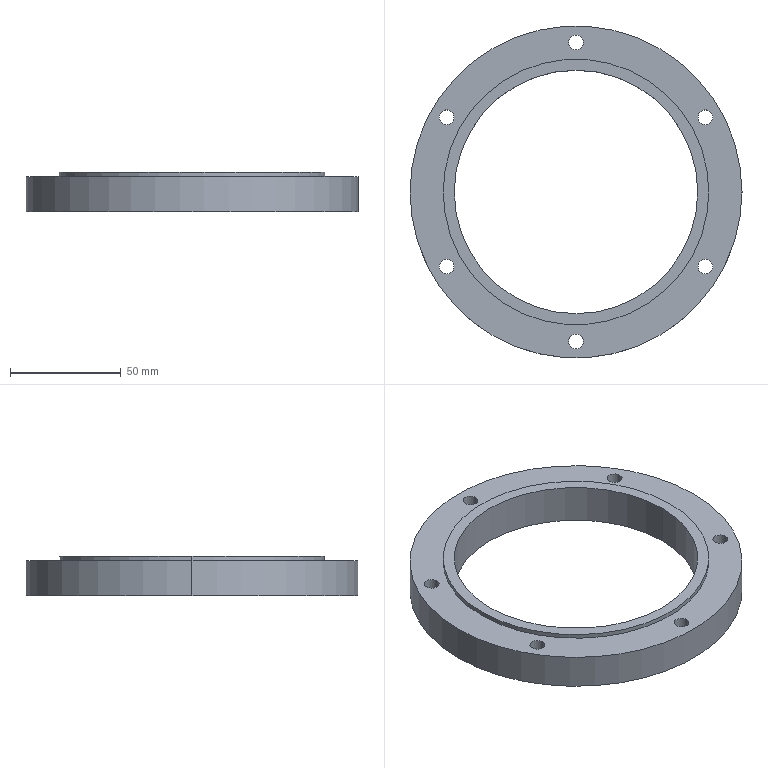Part | SolidWorks | features Extrusion 1, ICE 1 | 1 solid | 21 faces | box 150 x 150 x 18 mm | volume 130969 mm3 | cylinder 18 | plane 3 | commonest cylinder face diameters 6.65 x12 110 x2 120 x2 150 x2
STEP:
#1=CARTESIAN_POINT('',(60.,0.,18.));
#2=VERTEX_POINT('',#1);
#3=CARTESIAN_POINT('',(-60.,0.,18.));
#4=VERTEX_POINT('',#3);
#5=CARTESIAN_POINT('',(0.,0.,18.));
#6=DIRECTION('',(0.,0.,1.));
#7=DIRECTION('',(1.,0.,0.));
#8=AXIS2_PLACEMENT_3D('',#5,#6,#7);
#9=CIRCLE('',#8,60.);
#10=EDGE_CURVE('',#2,#4,#9,.T.);
#11=ORIENTED_EDGE('',*,*,#10,.F.);
#12=CARTESIAN_POINT('',(60.,0.,16.));
#13=VERTEX_POINT('',#12);
#14=CARTESIAN_POINT('',(60.,0.,18.));
#15=DIRECTION('',(0.,0.,-1.));
#16=VECTOR('',#15,1000.);
#17=LINE('',#14,#16);
#18=EDGE_CURVE('',#2,#13,#17,.T.);
#19=ORIENTED_EDGE('',*,*,#18,.T.);
#20=CARTESIAN_POINT('',(-60.,0.,16.));
#21=VERTEX_POINT('',#20);
#22=CARTESIAN_POINT('',(0.,0.,16.));
#23=DIRECTION('',(0.,0.,1.));
#24=DIRECTION('',(1.,0.,0.));
#25=AXIS2_PLACEMENT_3D('',#22,#23,#24);
#26=CIRCLE('',#25,60.);
#27=EDGE_CURVE('',#13,#21,#26,.T.);
#28=ORIENTED_EDGE('',*,*,#27,.T.);
#29=CARTESIAN_POINT('',(-60.,0.,18.));
#30=DIRECTION('',(0.,0.,-1.));
#31=VECTOR('',#30,1000.);
#32=LINE('',#29,#31);
#33=EDGE_CURVE('',#4,#21,#32,.T.);
#34=ORIENTED_EDGE('',*,*,#33,.F.);
#35=EDGE_LOOP('',(#11,#19,#28,#34));
#36=FACE_OUTER_BOUND('',#35,.T.);
#37=CARTESIAN_POINT('',(0.,0.,18.));
#38=DIRECTION('',(0.,0.,-1.));
#39=DIRECTION('',(-1.,0.,0.));
#40=AXIS2_PLACEMENT_3D('',#37,#38,#39);
#41=CYLINDRICAL_SURFACE('',#40,60.);
#42=ADVANCED_FACE('',(#36),#41,.T.);
#43=CARTESIAN_POINT('',(-61.782,33.75,16.));
#44=VERTEX_POINT('',#43);
#45=CARTESIAN_POINT('',(-55.132,33.75,16.));
#46=VERTEX_POINT('',#45);
#47=CARTESIAN_POINT('',(-58.457,33.75,16.));
#48=DIRECTION('',(0.,0.,1.));
#49=DIRECTION('',(1.,0.,0.));
#50=AXIS2_PLACEMENT_3D('',#47,#48,#49);
#51=CIRCLE('',#50,3.325);
#52=EDGE_CURVE('',#44,#46,#51,.T.);
#53=ORIENTED_EDGE('',*,*,#52,.T.);
#54=CARTESIAN_POINT('',(-55.132,33.75,0.));
#55=VERTEX_POINT('',#54);
#56=CARTESIAN_POINT('',(-55.132,33.75,16.));
#57=DIRECTION('',(0.,0.,-1.));
#58=VECTOR('',#57,1000.);
#59=LINE('',#56,#58);
#60=EDGE_CURVE('',#46,#55,#59,.T.);
#61=ORIENTED_EDGE('',*,*,#60,.T.);
#62=CARTESIAN_POINT('',(-61.782,33.75,0.));
#63=VERTEX_POINT('',#62);
#64=CARTESIAN_POINT('',(-58.457,33.75,0.));
#65=DIRECTION('',(0.,0.,1.));
#66=DIRECTION('',(1.,0.,0.));
#67=AXIS2_PLACEMENT_3D('',#64,#65,#66);
#68=CIRCLE('',#67,3.325);
#69=EDGE_CURVE('',#63,#55,#68,.T.);
#70=ORIENTED_EDGE('',*,*,#69,.F.);
#71=CARTESIAN_POINT('',(-61.782,33.75,16.));
#72=DIRECTION('',(0.,0.,-1.));
#73=VECTOR('',#72,1000.);
#74=LINE('',#71,#73);
#75=EDGE_CURVE('',#44,#63,#74,.T.);
#76=ORIENTED_EDGE('',*,*,#75,.F.);
#77=EDGE_LOOP('',(#53,#61,#70,#76));
#78=FACE_OUTER_BOUND('',#77,.T.);
#79=CARTESIAN_POINT('',(-58.457,33.75,16.));
#80=DIRECTION('',(0.,0.,-1.));
#81=DIRECTION('',(-1.,0.,0.));
#82=AXIS2_PLACEMENT_3D('',#79,#80,#81);
#83=CYLINDRICAL_SURFACE('',#82,3.325);
#84=ADVANCED_FACE('',(#78),#83,.F.);
#85=CARTESIAN_POINT('',(-61.782,-33.75,16.));
#86=VERTEX_POINT('',#85);
#87=CARTESIAN_POINT('',(-55.132,-33.75,16.));
#88=VERTEX_POINT('',#87);
#89=CARTESIAN_POINT('',(-58.457,-33.75,16.));
#90=DIRECTION('',(0.,0.,1.));
#91=DIRECTION('',(1.,0.,0.));
#92=AXIS2_PLACEMENT_3D('',#89,#90,#91);
#93=CIRCLE('',#92,3.325);
#94=EDGE_CURVE('',#86,#88,#93,.T.);
#95=ORIENTED_EDGE('',*,*,#94,.T.);
#96=CARTESIAN_POINT('',(-55.132,-33.75,0.));
#97=VERTEX_POINT('',#96);
#98=CARTESIAN_POINT('',(-55.132,-33.75,16.));
#99=DIRECTION('',(0.,0.,-1.));
#100=VECTOR('',#99,1000.);
#101=LINE('',#98,#100);
#102=EDGE_CURVE('',#88,#97,#101,.T.);
#103=ORIENTED_EDGE('',*,*,#102,.T.);
#104=CARTESIAN_POINT('',(-61.782,-33.75,0.));
#105=VERTEX_POINT('',#104);
#106=CARTESIAN_POINT('',(-58.457,-33.75,0.));
#107=DIRECTION('',(0.,0.,1.));
#108=DIRECTION('',(1.,0.,0.));
#109=AXIS2_PLACEMENT_3D('',#106,#107,#108);
#110=CIRCLE('',#109,3.325);
#111=EDGE_CURVE('',#105,#97,#110,.T.);
#112=ORIENTED_EDGE('',*,*,#111,.F.);
#113=CARTESIAN_POINT('',(-61.782,-33.75,16.));
#114=DIRECTION('',(0.,0.,-1.));
#115=VECTOR('',#114,1000.);
#116=LINE('',#113,#115);
#117=EDGE_CURVE('',#86,#105,#116,.T.);
#118=ORIENTED_EDGE('',*,*,#117,.F.);
#119=EDGE_LOOP('',(#95,#103,#112,#118));
#120=FACE_OUTER_BOUND('',#119,.T.);
#121=CARTESIAN_POINT('',(-58.457,-33.75,16.));
#122=DIRECTION('',(0.,0.,-1.));
#123=DIRECTION('',(-1.,0.,0.));
#124=AXIS2_PLACEMENT_3D('',#121,#122,#123);
#125=CYLINDRICAL_SURFACE('',#124,3.325);
#126=ADVANCED_FACE('',(#120),#125,.F.);
#127=CARTESIAN_POINT('',(-3.325,-67.5,16.));
#128=VERTEX_POINT('',#127);
#129=CARTESIAN_POINT('',(3.325,-67.5,16.));
#130=VERTEX_POINT('',#129);
#131=CARTESIAN_POINT('',(0.,-67.5,16.));
#132=DIRECTION('',(0.,0.,1.));
#133=DIRECTION('',(1.,0.,0.));
#134=AXIS2_PLACEMENT_3D('',#131,#132,#133);
#135=CIRCLE('',#134,3.325);
#136=EDGE_CURVE('',#128,#130,#135,.T.);
#137=ORIENTED_EDGE('',*,*,#136,.T.);
#138=CARTESIAN_POINT('',(3.325,-67.5,0.));
#139=VERTEX_POINT('',#138);
#140=CARTESIAN_POINT('',(3.325,-67.5,16.));
#141=DIRECTION('',(0.,0.,-1.));
#142=VECTOR('',#141,1000.);
#143=LINE('',#140,#142);
#144=EDGE_CURVE('',#130,#139,#143,.T.);
#145=ORIENTED_EDGE('',*,*,#144,.T.);
#146=CARTESIAN_POINT('',(-3.325,-67.5,0.));
#147=VERTEX_POINT('',#146);
#148=CARTESIAN_POINT('',(0.,-67.5,0.));
#149=DIRECTION('',(0.,0.,1.));
#150=DIRECTION('',(1.,0.,0.));
#151=AXIS2_PLACEMENT_3D('',#148,#149,#150);
#152=CIRCLE('',#151,3.325);
#153=EDGE_CURVE('',#147,#139,#152,.T.);
#154=ORIENTED_EDGE('',*,*,#153,.F.);
#155=CARTESIAN_POINT('',(-3.325,-67.5,16.));
#156=DIRECTION('',(0.,0.,-1.));
#157=VECTOR('',#156,1000.);
#158=LINE('',#155,#157);
#159=EDGE_CURVE('',#128,#147,#158,.T.);
#160=ORIENTED_EDGE('',*,*,#159,.F.);
#161=EDGE_LOOP('',(#137,#145,#154,#160));
#162=FACE_OUTER_BOUND('',#161,.T.);
#163=CARTESIAN_POINT('',(0.,-67.5,16.));
#164=DIRECTION('',(0.,0.,-1.));
#165=DIRECTION('',(-1.,0.,0.));
#166=AXIS2_PLACEMENT_3D('',#163,#164,#165);
#167=CYLINDRICAL_SURFACE('',#166,3.325);
#168=ADVANCED_FACE('',(#162),#167,.F.);
#169=CARTESIAN_POINT('',(55.132,-33.75,16.));
#170=VERTEX_POINT('',#169);
#171=CARTESIAN_POINT('',(61.782,-33.75,16.));
#172=VERTEX_POINT('',#171);
#173=CARTESIAN_POINT('',(58.457,-33.75,16.));
#174=DIRECTION('',(0.,0.,1.));
#175=DIRECTION('',(1.,0.,0.));
#176=AXIS2_PLACEMENT_3D('',#173,#174,#175);
#177=CIRCLE('',#176,3.325);
#178=EDGE_CURVE('',#170,#172,#177,.T.);
#179=ORIENTED_EDGE('',*,*,#178,.T.);
#180=CARTESIAN_POINT('',(61.782,-33.75,0.));
#181=VERTEX_POINT('',#180);
#182=CARTESIAN_POINT('',(61.782,-33.75,16.));
#183=DIRECTION('',(0.,0.,-1.));
#184=VECTOR('',#183,1000.);
#185=LINE('',#182,#184);
#186=EDGE_CURVE('',#172,#181,#185,.T.);
#187=ORIENTED_EDGE('',*,*,#186,.T.);
#188=CARTESIAN_POINT('',(55.132,-33.75,0.));
#189=VERTEX_POINT('',#188);
#190=CARTESIAN_POINT('',(58.457,-33.75,0.));
#191=DIRECTION('',(0.,0.,1.));
#192=DIRECTION('',(1.,0.,0.));
#193=AXIS2_PLACEMENT_3D('',#190,#191,#192);
#194=CIRCLE('',#193,3.325);
#195=EDGE_CURVE('',#189,#181,#194,.T.);
#196=ORIENTED_EDGE('',*,*,#195,.F.);
#197=CARTESIAN_POINT('',(55.132,-33.75,16.));
#198=DIRECTION('',(0.,0.,-1.));
#199=VECTOR('',#198,1000.);
#200=LINE('',#197,#199);
#201=EDGE_CURVE('',#170,#189,#200,.T.);
#202=ORIENTED_EDGE('',*,*,#201,.F.);
#203=EDGE_LOOP('',(#179,#187,#196,#202));
#204=FACE_OUTER_BOUND('',#203,.T.);
#205=CARTESIAN_POINT('',(58.457,-33.75,16.));
#206=DIRECTION('',(0.,0.,-1.));
#207=DIRECTION('',(-1.,0.,0.));
#208=AXIS2_PLACEMENT_3D('',#205,#206,#207);
#209=CYLINDRICAL_SURFACE('',#208,3.325);
#210=ADVANCED_FACE('',(#204),#209,.F.);
#211=CARTESIAN_POINT('',(55.132,33.75,16.));
#212=VERTEX_POINT('',#211);
#213=CARTESIAN_POINT('',(61.782,33.75,16.));
#214=VERTEX_POINT('',#213);
#215=CARTESIAN_POINT('',(58.457,33.75,16.));
#216=DIRECTION('',(0.,0.,1.));
#217=DIRECTION('',(1.,0.,0.));
#218=AXIS2_PLACEMENT_3D('',#215,#216,#217);
#219=CIRCLE('',#218,3.325);
#220=EDGE_CURVE('',#212,#214,#219,.T.);
#221=ORIENTED_EDGE('',*,*,#220,.T.);
#222=CARTESIAN_POINT('',(61.782,33.75,0.));
#223=VERTEX_POINT('',#222);
#224=CARTESIAN_POINT('',(61.782,33.75,16.));
#225=DIRECTION('',(0.,0.,-1.));
#226=VECTOR('',#225,1000.);
#227=LINE('',#224,#226);
#228=EDGE_CURVE('',#214,#223,#227,.T.);
#229=ORIENTED_EDGE('',*,*,#228,.T.);
#230=CARTESIAN_POINT('',(55.132,33.75,0.));
#231=VERTEX_POINT('',#230);
#232=CARTESIAN_POINT('',(58.457,33.75,0.));
#233=DIRECTION('',(0.,0.,1.));
#234=DIRECTION('',(1.,0.,0.));
#235=AXIS2_PLACEMENT_3D('',#232,#233,#234);
#236=CIRCLE('',#235,3.325);
#237=EDGE_CURVE('',#231,#223,#236,.T.);
#238=ORIENTED_EDGE('',*,*,#237,.F.);
#239=CARTESIAN_POINT('',(55.132,33.75,16.));
#240=DIRECTION('',(0.,0.,-1.));
#241=VECTOR('',#240,1000.);
#242=LINE('',#239,#241);
#243=EDGE_CURVE('',#212,#231,#242,.T.);
#244=ORIENTED_EDGE('',*,*,#243,.F.);
#245=EDGE_LOOP('',(#221,#229,#238,#244));
#246=FACE_OUTER_BOUND('',#245,.T.);
#247=CARTESIAN_POINT('',(58.457,33.75,16.));
#248=DIRECTION('',(0.,0.,-1.));
#249=DIRECTION('',(-1.,0.,0.));
#250=AXIS2_PLACEMENT_3D('',#247,#248,#249);
#251=CYLINDRICAL_SURFACE('',#250,3.325);
#252=ADVANCED_FACE('',(#246),#251,.F.);
#253=CARTESIAN_POINT('',(-3.325,67.5,16.));
#254=VERTEX_POINT('',#253);
#255=CARTESIAN_POINT('',(3.325,67.5,16.));
#256=VERTEX_POINT('',#255);
#257=CARTESIAN_POINT('',(0.,67.5,16.));
#258=DIRECTION('',(0.,0.,1.));
#259=DIRECTION('',(1.,0.,0.));
#260=AXIS2_PLACEMENT_3D('',#257,#258,#259);
#261=CIRCLE('',#260,3.325);
#262=EDGE_CURVE('',#254,#256,#261,.T.);
#263=ORIENTED_EDGE('',*,*,#262,.T.);
#264=CARTESIAN_POINT('',(3.325,67.5,0.));
#265=VERTEX_POINT('',#264);
#266=CARTESIAN_POINT('',(3.325,67.5,16.));
#267=DIRECTION('',(0.,0.,-1.));
#268=VECTOR('',#267,1000.);
#269=LINE('',#266,#268);
#270=EDGE_CURVE('',#256,#265,#269,.T.);
#271=ORIENTED_EDGE('',*,*,#270,.T.);
#272=CARTESIAN_POINT('',(-3.325,67.5,0.));
#273=VERTEX_POINT('',#272);
#274=CARTESIAN_POINT('',(0.,67.5,0.));
#275=DIRECTION('',(0.,0.,1.));
#276=DIRECTION('',(1.,0.,0.));
#277=AXIS2_PLACEMENT_3D('',#274,#275,#276);
#278=CIRCLE('',#277,3.325);
#279=EDGE_CURVE('',#273,#265,#278,.T.);
#280=ORIENTED_EDGE('',*,*,#279,.F.);
#281=CARTESIAN_POINT('',(-3.325,67.5,16.));
#282=DIRECTION('',(0.,0.,-1.));
#283=VECTOR('',#282,1000.);
#284=LINE('',#281,#283);
#285=EDGE_CURVE('',#254,#273,#284,.T.);
#286=ORIENTED_EDGE('',*,*,#285,.F.);
#287=EDGE_LOOP('',(#263,#271,#280,#286));
#288=FACE_OUTER_BOUND('',#287,.T.);
#289=CARTESIAN_POINT('',(0.,67.5,16.));
#290=DIRECTION('',(0.,0.,-1.));
#291=DIRECTION('',(-1.,0.,0.));
#292=AXIS2_PLACEMENT_3D('',#289,#290,#291);
#293=CYLINDRICAL_SURFACE('',#292,3.325);
#294=ADVANCED_FACE('',(#288),#293,.F.);
#295=CARTESIAN_POINT('',(-55.,0.,18.));
#296=VERTEX_POINT('',#295);
#297=CARTESIAN_POINT('',(55.,0.,18.));
#298=VERTEX_POINT('',#297);
#299=CARTESIAN_POINT('',(0.,0.,18.));
#300=DIRECTION('',(0.,0.,1.));
#301=DIRECTION('',(1.,0.,0.));
#302=AXIS2_PLACEMENT_3D('',#299,#300,#301);
#303=CIRCLE('',#302,55.);
#304=EDGE_CURVE('',#296,#298,#303,.T.);
#305=ORIENTED_EDGE('',*,*,#304,.T.);
#306=CARTESIAN_POINT('',(55.,0.,0.));
#307=VERTEX_POINT('',#306);
#308=CARTESIAN_POINT('',(55.,0.,16.));
#309=DIRECTION('',(0.,0.,-1.));
#310=VECTOR('',#309,1000.);
#311=LINE('',#308,#310);
#312=EDGE_CURVE('',#298,#307,#311,.T.);
#313=ORIENTED_EDGE('',*,*,#312,.T.);
#314=CARTESIAN_POINT('',(-55.,0.,0.));
#315=VERTEX_POINT('',#314);
#316=CARTESIAN_POINT('',(0.,0.,0.));
#317=DIRECTION('',(0.,0.,1.));
#318=DIRECTION('',(1.,0.,0.));
#319=AXIS2_PLACEMENT_3D('',#316,#317,#318);
#320=CIRCLE('',#319,55.);
#321=EDGE_CURVE('',#315,#307,#320,.T.);
#322=ORIENTED_EDGE('',*,*,#321,.F.);
#323=CARTESIAN_POINT('',(-55.,0.,16.));
#324=DIRECTION('',(0.,0.,-1.));
#325=VECTOR('',#324,1000.);
#326=LINE('',#323,#325);
#327=EDGE_CURVE('',#296,#315,#326,.T.);
#328=ORIENTED_EDGE('',*,*,#327,.F.);
#329=EDGE_LOOP('',(#305,#313,#322,#328));
#330=FACE_OUTER_BOUND('',#329,.T.);
#331=CARTESIAN_POINT('',(0.,0.,16.));
#332=DIRECTION('',(0.,0.,-1.));
#333=DIRECTION('',(-1.,0.,0.));
#334=AXIS2_PLACEMENT_3D('',#331,#332,#333);
#335=CYLINDRICAL_SURFACE('',#334,55.);
#336=ADVANCED_FACE('',(#330),#335,.F.);
#337=CARTESIAN_POINT('',(75.,0.,16.));
#338=VERTEX_POINT('',#337);
#339=CARTESIAN_POINT('',(-75.,0.,16.));
#340=VERTEX_POINT('',#339);
#341=CARTESIAN_POINT('',(0.,0.,16.));
#342=DIRECTION('',(0.,0.,1.));
#343=DIRECTION('',(1.,0.,0.));
#344=AXIS2_PLACEMENT_3D('',#341,#342,#343);
#345=CIRCLE('',#344,75.);
#346=EDGE_CURVE('',#338,#340,#345,.T.);
#347=ORIENTED_EDGE('',*,*,#346,.F.);
#348=CARTESIAN_POINT('',(75.,0.,0.));
#349=VERTEX_POINT('',#348);
#350=CARTESIAN_POINT('',(75.,0.,16.));
#351=DIRECTION('',(0.,0.,-1.));
#352=VECTOR('',#351,1000.);
#353=LINE('',#350,#352);
#354=EDGE_CURVE('',#338,#349,#353,.T.);
#355=ORIENTED_EDGE('',*,*,#354,.T.);
#356=CARTESIAN_POINT('',(-75.,0.,0.));
#357=VERTEX_POINT('',#356);
#358=CARTESIAN_POINT('',(0.,0.,0.));
#359=DIRECTION('',(0.,0.,1.));
#360=DIRECTION('',(1.,0.,0.));
#361=AXIS2_PLACEMENT_3D('',#358,#359,#360);
#362=CIRCLE('',#361,75.);
#363=EDGE_CURVE('',#349,#357,#362,.T.);
#364=ORIENTED_EDGE('',*,*,#363,.T.);
#365=CARTESIAN_POINT('',(-75.,0.,16.));
#366=DIRECTION('',(0.,0.,-1.));
#367=VECTOR('',#366,1000.);
#368=LINE('',#365,#367);
#369=EDGE_CURVE('',#340,#357,#368,.T.);
#370=ORIENTED_EDGE('',*,*,#369,.F.);
#371=EDGE_LOOP('',(#347,#355,#364,#370));
#372=FACE_OUTER_BOUND('',#371,.T.);
#373=CARTESIAN_POINT('',(0.,0.,16.));
#374=DIRECTION('',(0.,0.,-1.));
#375=DIRECTION('',(-1.,0.,0.));
#376=AXIS2_PLACEMENT_3D('',#373,#374,#375);
#377=CYLINDRICAL_SURFACE('',#376,75.);
#378=ADVANCED_FACE('',(#372),#377,.T.);
#379=ORIENTED_EDGE('',*,*,#52,.F.);
#380=CARTESIAN_POINT('',(-58.457,33.75,16.));
#381=DIRECTION('',(0.,0.,1.));
#382=DIRECTION('',(1.,0.,0.));
#383=AXIS2_PLACEMENT_3D('',#380,#381,#382);
#384=CIRCLE('',#383,3.325);
#385=EDGE_CURVE('',#46,#44,#384,.T.);
#386=ORIENTED_EDGE('',*,*,#385,.F.);
#387=EDGE_LOOP('',(#379,#386));
#388=FACE_BOUND('',#387,.T.);
#389=ORIENTED_EDGE('',*,*,#136,.F.);
#390=CARTESIAN_POINT('',(0.,-67.5,16.));
#391=DIRECTION('',(0.,0.,1.));
#392=DIRECTION('',(1.,0.,0.));
#393=AXIS2_PLACEMENT_3D('',#390,#391,#392);
#394=CIRCLE('',#393,3.325);
#395=EDGE_CURVE('',#130,#128,#394,.T.);
#396=ORIENTED_EDGE('',*,*,#395,.F.);
#397=EDGE_LOOP('',(#389,#396));
#398=FACE_BOUND('',#397,.T.);
#399=ORIENTED_EDGE('',*,*,#220,.F.);
#400=CARTESIAN_POINT('',(58.457,33.75,16.));
#401=DIRECTION('',(0.,0.,1.));
#402=DIRECTION('',(1.,0.,0.));
#403=AXIS2_PLACEMENT_3D('',#400,#401,#402);
#404=CIRCLE('',#403,3.325);
#405=EDGE_CURVE('',#214,#212,#404,.T.);
#406=ORIENTED_EDGE('',*,*,#405,.F.);
#407=EDGE_LOOP('',(#399,#406));
#408=FACE_BOUND('',#407,.T.);
#409=CARTESIAN_POINT('',(0.,0.,16.));
#410=DIRECTION('',(0.,0.,1.));
#411=DIRECTION('',(1.,0.,0.));
#412=AXIS2_PLACEMENT_3D('',#409,#410,#411);
#413=CIRCLE('',#412,75.);
#414=EDGE_CURVE('',#340,#338,#413,.T.);
#415=ORIENTED_EDGE('',*,*,#414,.T.);
#416=ORIENTED_EDGE('',*,*,#346,.T.);
#417=EDGE_LOOP('',(#415,#416));
#418=FACE_OUTER_BOUND('',#417,.T.);
#419=ORIENTED_EDGE('',*,*,#262,.F.);
#420=CARTESIAN_POINT('',(0.,67.5,16.));
#421=DIRECTION('',(0.,0.,1.));
#422=DIRECTION('',(1.,0.,0.));
#423=AXIS2_PLACEMENT_3D('',#420,#421,#422);
#424=CIRCLE('',#423,3.325);
#425=EDGE_CURVE('',#256,#254,#424,.T.);
#426=ORIENTED_EDGE('',*,*,#425,.F.);
#427=EDGE_LOOP('',(#419,#426));
#428=FACE_BOUND('',#427,.T.);
#429=ORIENTED_EDGE('',*,*,#178,.F.);
#430=CARTESIAN_POINT('',(58.457,-33.75,16.));
#431=DIRECTION('',(0.,0.,1.));
#432=DIRECTION('',(1.,0.,0.));
#433=AXIS2_PLACEMENT_3D('',#430,#431,#432);
#434=CIRCLE('',#433,3.325);
#435=EDGE_CURVE('',#172,#170,#434,.T.);
#436=ORIENTED_EDGE('',*,*,#435,.F.);
#437=EDGE_LOOP('',(#429,#436));
#438=FACE_BOUND('',#437,.T.);
#439=ORIENTED_EDGE('',*,*,#94,.F.);
#440=CARTESIAN_POINT('',(-58.457,-33.75,16.));
#441=DIRECTION('',(0.,0.,1.));
#442=DIRECTION('',(1.,0.,0.));
#443=AXIS2_PLACEMENT_3D('',#440,#441,#442);
#444=CIRCLE('',#443,3.325);
#445=EDGE_CURVE('',#88,#86,#444,.T.);
#446=ORIENTED_EDGE('',*,*,#445,.F.);
#447=EDGE_LOOP('',(#439,#446));
#448=FACE_BOUND('',#447,.T.);
#449=CARTESIAN_POINT('',(0.,0.,16.));
#450=DIRECTION('',(0.,0.,1.));
#451=DIRECTION('',(1.,0.,0.));
#452=AXIS2_PLACEMENT_3D('',#449,#450,#451);
#453=CIRCLE('',#452,60.);
#454=EDGE_CURVE('',#21,#13,#453,.T.);
#455=ORIENTED_EDGE('',*,*,#454,.F.);
#456=ORIENTED_EDGE('',*,*,#27,.F.);
#457=EDGE_LOOP('',(#455,#456));
#458=FACE_BOUND('',#457,.T.);
#459=CARTESIAN_POINT('',(0.,0.,16.));
#460=DIRECTION('',(0.,0.,1.));
#461=DIRECTION('',(1.,0.,0.));
#462=AXIS2_PLACEMENT_3D('',#459,#460,#461);
#463=PLANE('',#462);
#464=ADVANCED_FACE('',(#388,#398,#408,#418,#428,#438,#448,#458),#463,.T.);
#465=CARTESIAN_POINT('',(0.,0.,0.));
#466=DIRECTION('',(0.,0.,1.));
#467=DIRECTION('',(1.,0.,0.));
#468=AXIS2_PLACEMENT_3D('',#465,#466,#467);
#469=CIRCLE('',#468,75.);
#470=EDGE_CURVE('',#357,#349,#469,.T.);
#471=ORIENTED_EDGE('',*,*,#470,.F.);
#472=ORIENTED_EDGE('',*,*,#363,.F.);
#473=EDGE_LOOP('',(#471,#472));
#474=FACE_OUTER_BOUND('',#473,.T.);
#475=ORIENTED_EDGE('',*,*,#321,.T.);
#476=CARTESIAN_POINT('',(0.,0.,0.));
#477=DIRECTION('',(0.,0.,1.));
#478=DIRECTION('',(1.,0.,0.));
#479=AXIS2_PLACEMENT_3D('',#476,#477,#478);
#480=CIRCLE('',#479,55.);
#481=EDGE_CURVE('',#307,#315,#480,.T.);
#482=ORIENTED_EDGE('',*,*,#481,.T.);
#483=EDGE_LOOP('',(#475,#482));
#484=FACE_BOUND('',#483,.T.);
#485=ORIENTED_EDGE('',*,*,#279,.T.);
#486=CARTESIAN_POINT('',(0.,67.5,0.));
#487=DIRECTION('',(0.,0.,1.));
#488=DIRECTION('',(1.,0.,0.));
#489=AXIS2_PLACEMENT_3D('',#486,#487,#488);
#490=CIRCLE('',#489,3.325);
#491=EDGE_CURVE('',#265,#273,#490,.T.);
#492=ORIENTED_EDGE('',*,*,#491,.T.);
#493=EDGE_LOOP('',(#485,#492));
#494=FACE_BOUND('',#493,.T.);
#495=ORIENTED_EDGE('',*,*,#237,.T.);
#496=CARTESIAN_POINT('',(58.457,33.75,0.));
#497=DIRECTION('',(0.,0.,1.));
#498=DIRECTION('',(1.,0.,0.));
#499=AXIS2_PLACEMENT_3D('',#496,#497,#498);
#500=CIRCLE('',#499,3.325);
#501=EDGE_CURVE('',#223,#231,#500,.T.);
#502=ORIENTED_EDGE('',*,*,#501,.T.);
#503=EDGE_LOOP('',(#495,#502));
#504=FACE_BOUND('',#503,.T.);
#505=ORIENTED_EDGE('',*,*,#195,.T.);
#506=CARTESIAN_POINT('',(58.457,-33.75,0.));
#507=DIRECTION('',(0.,0.,1.));
#508=DIRECTION('',(1.,0.,0.));
#509=AXIS2_PLACEMENT_3D('',#506,#507,#508);
#510=CIRCLE('',#509,3.325);
#511=EDGE_CURVE('',#181,#189,#510,.T.);
#512=ORIENTED_EDGE('',*,*,#511,.T.);
#513=EDGE_LOOP('',(#505,#512));
#514=FACE_BOUND('',#513,.T.);
#515=ORIENTED_EDGE('',*,*,#153,.T.);
#516=CARTESIAN_POINT('',(0.,-67.5,0.));
#517=DIRECTION('',(0.,0.,1.));
#518=DIRECTION('',(1.,0.,0.));
#519=AXIS2_PLACEMENT_3D('',#516,#517,#518);
#520=CIRCLE('',#519,3.325);
#521=EDGE_CURVE('',#139,#147,#520,.T.);
#522=ORIENTED_EDGE('',*,*,#521,.T.);
#523=EDGE_LOOP('',(#515,#522));
#524=FACE_BOUND('',#523,.T.);
#525=ORIENTED_EDGE('',*,*,#111,.T.);
#526=CARTESIAN_POINT('',(-58.457,-33.75,0.));
#527=DIRECTION('',(0.,0.,1.));
#528=DIRECTION('',(1.,0.,0.));
#529=AXIS2_PLACEMENT_3D('',#526,#527,#528);
#530=CIRCLE('',#529,3.325);
#531=EDGE_CURVE('',#97,#105,#530,.T.);
#532=ORIENTED_EDGE('',*,*,#531,.T.);
#533=EDGE_LOOP('',(#525,#532));
#534=FACE_BOUND('',#533,.T.);
#535=ORIENTED_EDGE('',*,*,#69,.T.);
#536=CARTESIAN_POINT('',(-58.457,33.75,0.));
#537=DIRECTION('',(0.,0.,1.));
#538=DIRECTION('',(1.,0.,0.));
#539=AXIS2_PLACEMENT_3D('',#536,#537,#538);
#540=CIRCLE('',#539,3.325);
#541=EDGE_CURVE('',#55,#63,#540,.T.);
#542=ORIENTED_EDGE('',*,*,#541,.T.);
#543=EDGE_LOOP('',(#535,#542));
#544=FACE_BOUND('',#543,.T.);
#545=CARTESIAN_POINT('',(0.,0.,0.));
#546=DIRECTION('',(0.,0.,1.));
#547=DIRECTION('',(1.,0.,0.));
#548=AXIS2_PLACEMENT_3D('',#545,#546,#547);
#549=PLANE('',#548);
#550=ADVANCED_FACE('',(#474,#484,#494,#504,#514,#524,#534,#544),#549,.F.);
#551=ORIENTED_EDGE('',*,*,#354,.F.);
#552=ORIENTED_EDGE('',*,*,#414,.F.);
#553=ORIENTED_EDGE('',*,*,#369,.T.);
#554=ORIENTED_EDGE('',*,*,#470,.T.);
#555=EDGE_LOOP('',(#551,#552,#553,#554));
#556=FACE_OUTER_BOUND('',#555,.T.);
#557=CARTESIAN_POINT('',(0.,0.,16.));
#558=DIRECTION('',(0.,0.,-1.));
#559=DIRECTION('',(-1.,0.,0.));
#560=AXIS2_PLACEMENT_3D('',#557,#558,#559);
#561=CYLINDRICAL_SURFACE('',#560,75.);
#562=ADVANCED_FACE('',(#556),#561,.T.);
#563=ORIENTED_EDGE('',*,*,#312,.F.);
#564=CARTESIAN_POINT('',(0.,0.,18.));
#565=DIRECTION('',(0.,0.,1.));
#566=DIRECTION('',(1.,0.,0.));
#567=AXIS2_PLACEMENT_3D('',#564,#565,#566);
#568=CIRCLE('',#567,55.);
#569=EDGE_CURVE('',#298,#296,#568,.T.);
#570=ORIENTED_EDGE('',*,*,#569,.T.);
#571=ORIENTED_EDGE('',*,*,#327,.T.);
#572=ORIENTED_EDGE('',*,*,#481,.F.);
#573=EDGE_LOOP('',(#563,#570,#571,#572));
#574=FACE_OUTER_BOUND('',#573,.T.);
#575=CARTESIAN_POINT('',(0.,0.,16.));
#576=DIRECTION('',(0.,0.,-1.));
#577=DIRECTION('',(-1.,0.,0.));
#578=AXIS2_PLACEMENT_3D('',#575,#576,#577);
#579=CYLINDRICAL_SURFACE('',#578,55.);
#580=ADVANCED_FACE('',(#574),#579,.F.);
#581=ORIENTED_EDGE('',*,*,#270,.F.);
#582=ORIENTED_EDGE('',*,*,#425,.T.);
#583=ORIENTED_EDGE('',*,*,#285,.T.);
#584=ORIENTED_EDGE('',*,*,#491,.F.);
#585=EDGE_LOOP('',(#581,#582,#583,#584));
#586=FACE_OUTER_BOUND('',#585,.T.);
#587=CARTESIAN_POINT('',(0.,67.5,16.));
#588=DIRECTION('',(0.,0.,-1.));
#589=DIRECTION('',(-1.,0.,0.));
#590=AXIS2_PLACEMENT_3D('',#587,#588,#589);
#591=CYLINDRICAL_SURFACE('',#590,3.325);
#592=ADVANCED_FACE('',(#586),#591,.F.);
#593=ORIENTED_EDGE('',*,*,#228,.F.);
#594=ORIENTED_EDGE('',*,*,#405,.T.);
#595=ORIENTED_EDGE('',*,*,#243,.T.);
#596=ORIENTED_EDGE('',*,*,#501,.F.);
#597=EDGE_LOOP('',(#593,#594,#595,#596));
#598=FACE_OUTER_BOUND('',#597,.T.);
#599=CARTESIAN_POINT('',(58.457,33.75,16.));
#600=DIRECTION('',(0.,0.,-1.));
#601=DIRECTION('',(-1.,0.,0.));
#602=AXIS2_PLACEMENT_3D('',#599,#600,#601);
#603=CYLINDRICAL_SURFACE('',#602,3.325);
#604=ADVANCED_FACE('',(#598),#603,.F.);
#605=ORIENTED_EDGE('',*,*,#186,.F.);
#606=ORIENTED_EDGE('',*,*,#435,.T.);
#607=ORIENTED_EDGE('',*,*,#201,.T.);
#608=ORIENTED_EDGE('',*,*,#511,.F.);
#609=EDGE_LOOP('',(#605,#606,#607,#608));
#610=FACE_OUTER_BOUND('',#609,.T.);
#611=CARTESIAN_POINT('',(58.457,-33.75,16.));
#612=DIRECTION('',(0.,0.,-1.));
#613=DIRECTION('',(-1.,0.,0.));
#614=AXIS2_PLACEMENT_3D('',#611,#612,#613);
#615=CYLINDRICAL_SURFACE('',#614,3.325);
#616=ADVANCED_FACE('',(#610),#615,.F.);
#617=ORIENTED_EDGE('',*,*,#144,.F.);
#618=ORIENTED_EDGE('',*,*,#395,.T.);
#619=ORIENTED_EDGE('',*,*,#159,.T.);
#620=ORIENTED_EDGE('',*,*,#521,.F.);
#621=EDGE_LOOP('',(#617,#618,#619,#620));
#622=FACE_OUTER_BOUND('',#621,.T.);
#623=CARTESIAN_POINT('',(0.,-67.5,16.));
#624=DIRECTION('',(0.,0.,-1.));
#625=DIRECTION('',(-1.,0.,0.));
#626=AXIS2_PLACEMENT_3D('',#623,#624,#625);
#627=CYLINDRICAL_SURFACE('',#626,3.325);
#628=ADVANCED_FACE('',(#622),#627,.F.);
#629=ORIENTED_EDGE('',*,*,#102,.F.);
#630=ORIENTED_EDGE('',*,*,#445,.T.);
#631=ORIENTED_EDGE('',*,*,#117,.T.);
#632=ORIENTED_EDGE('',*,*,#531,.F.);
#633=EDGE_LOOP('',(#629,#630,#631,#632));
#634=FACE_OUTER_BOUND('',#633,.T.);
#635=CARTESIAN_POINT('',(-58.457,-33.75,16.));
#636=DIRECTION('',(0.,0.,-1.));
#637=DIRECTION('',(-1.,0.,0.));
#638=AXIS2_PLACEMENT_3D('',#635,#636,#637);
#639=CYLINDRICAL_SURFACE('',#638,3.325);
#640=ADVANCED_FACE('',(#634),#639,.F.);
#641=ORIENTED_EDGE('',*,*,#60,.F.);
#642=ORIENTED_EDGE('',*,*,#385,.T.);
#643=ORIENTED_EDGE('',*,*,#75,.T.);
#644=ORIENTED_EDGE('',*,*,#541,.F.);
#645=EDGE_LOOP('',(#641,#642,#643,#644));
#646=FACE_OUTER_BOUND('',#645,.T.);
#647=CARTESIAN_POINT('',(-58.457,33.75,16.));
#648=DIRECTION('',(0.,0.,-1.));
#649=DIRECTION('',(-1.,0.,0.));
#650=AXIS2_PLACEMENT_3D('',#647,#648,#649);
#651=CYLINDRICAL_SURFACE('',#650,3.325);
#652=ADVANCED_FACE('',(#646),#651,.F.);
#653=CARTESIAN_POINT('',(0.,0.,18.));
#654=DIRECTION('',(0.,0.,1.));
#655=DIRECTION('',(1.,0.,0.));
#656=AXIS2_PLACEMENT_3D('',#653,#654,#655);
#657=CIRCLE('',#656,60.);
#658=EDGE_CURVE('',#4,#2,#657,.T.);
#659=ORIENTED_EDGE('',*,*,#658,.T.);
#660=ORIENTED_EDGE('',*,*,#10,.T.);
#661=EDGE_LOOP('',(#659,#660));
#662=FACE_OUTER_BOUND('',#661,.T.);
#663=ORIENTED_EDGE('',*,*,#304,.F.);
#664=ORIENTED_EDGE('',*,*,#569,.F.);
#665=EDGE_LOOP('',(#663,#664));
#666=FACE_BOUND('',#665,.T.);
#667=CARTESIAN_POINT('',(0.,0.,18.));
#668=DIRECTION('',(0.,0.,1.));
#669=DIRECTION('',(1.,0.,0.));
#670=AXIS2_PLACEMENT_3D('',#667,#668,#669);
#671=PLANE('',#670);
#672=ADVANCED_FACE('',(#662,#666),#671,.T.);
#673=ORIENTED_EDGE('',*,*,#18,.F.);
#674=ORIENTED_EDGE('',*,*,#658,.F.);
#675=ORIENTED_EDGE('',*,*,#33,.T.);
#676=ORIENTED_EDGE('',*,*,#454,.T.);
#677=EDGE_LOOP('',(#673,#674,#675,#676));
#678=FACE_OUTER_BOUND('',#677,.T.);
#679=CARTESIAN_POINT('',(0.,0.,18.));
#680=DIRECTION('',(0.,0.,-1.));
#681=DIRECTION('',(-1.,0.,0.));
#682=AXIS2_PLACEMENT_3D('',#679,#680,#681);
#683=CYLINDRICAL_SURFACE('',#682,60.);
#684=ADVANCED_FACE('',(#678),#683,.T.);
#685=CLOSED_SHELL('',(#42,#84,#126,#168,#210,#252,#294,#336,#378,#464,#550,#562,#580,#592,#604,#616,#628,#640,#652,#672,#684));
#686=MANIFOLD_SOLID_BREP('',#685);
#687=CARTESIAN_POINT('',(0.,0.,0.));
#688=DIRECTION('',(0.,0.,1.));
#689=DIRECTION('',(1.,0.,0.));
#690=AXIS2_PLACEMENT_3D('',#687,#688,#689);
#691=(LENGTH_UNIT()NAMED_UNIT(*)SI_UNIT(.MILLI.,.METRE.));
#692=UNCERTAINTY_MEASURE_WITH_UNIT(LENGTH_MEASURE(0.00001),#691,'','');
#693=(NAMED_UNIT(*)PLANE_ANGLE_UNIT()SI_UNIT($,.RADIAN.));
#694=(NAMED_UNIT(*)SI_UNIT($,.STERADIAN.)SOLID_ANGLE_UNIT());
#695=(GEOMETRIC_REPRESENTATION_CONTEXT(3)GLOBAL_UNCERTAINTY_ASSIGNED_CONTEXT((#692))GLOBAL_UNIT_ASSIGNED_CONTEXT((#691,#693,#694))REPRESENTATION_CONTEXT('',''));
#696=ADVANCED_BREP_SHAPE_REPRESENTATION('',(#686,#690),#695);